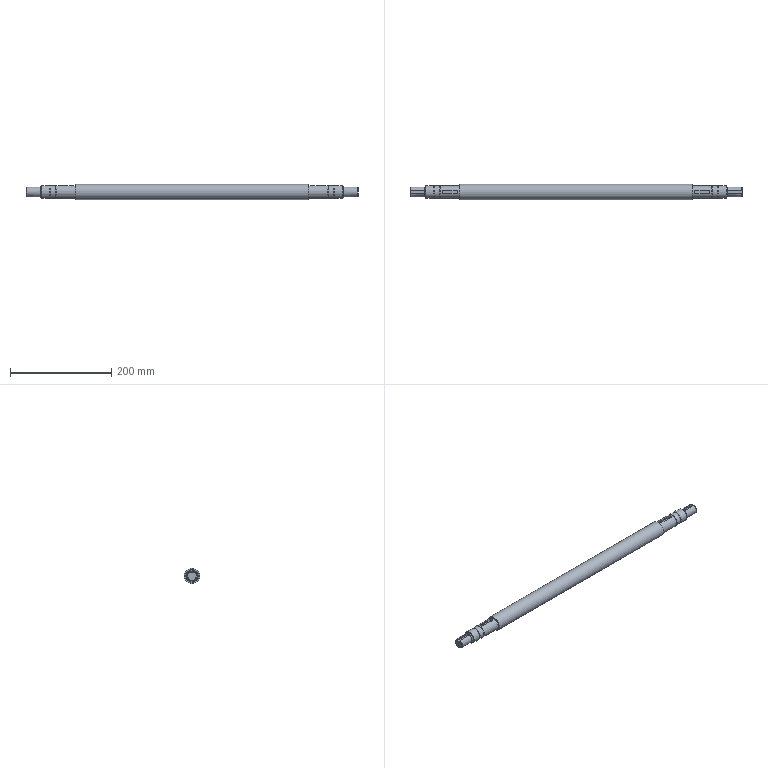Part | 2 solids | 52 faces | box 656 x 30.5 x 30.5 mm | volume 419502 mm3 | plane 27 | cylinder 19 | cone 4 | torus 2 | commonest cylinder face diameters 6 x6 23 x4 25 x4 19.5 x2 25.5 x2 30.5 x1
STEP:
#1=CARTESIAN_POINT('',(-538.673,-3091.93,7.953));
#2=VERTEX_POINT('',#1);
#3=CARTESIAN_POINT('',(-538.673,-3097.93,7.953));
#4=VERTEX_POINT('',#3);
#5=CARTESIAN_POINT('',(-538.673,-3094.93,0.));
#6=DIRECTION('',(-1.,0.,0.));
#7=DIRECTION('',(0.,0.,1.));
#8=AXIS2_PLACEMENT_3D('',#5,#6,#7);
#9=CIRCLE('',#8,8.5);
#10=EDGE_CURVE('',#2,#4,#9,.T.);
#11=ORIENTED_EDGE('',*,*,#10,.T.);
#12=CARTESIAN_POINT('',(-538.673,-3097.93,6.5));
#13=VERTEX_POINT('',#12);
#14=CARTESIAN_POINT('',(-538.673,-3097.93,15.));
#15=DIRECTION('',(0.,0.,-1.));
#16=VECTOR('',#15,1000.);
#17=LINE('',#14,#16);
#18=EDGE_CURVE('',#4,#13,#17,.T.);
#19=ORIENTED_EDGE('',*,*,#18,.T.);
#20=CARTESIAN_POINT('',(-538.673,-3091.93,6.5));
#21=VERTEX_POINT('',#20);
#22=CARTESIAN_POINT('',(-538.673,-3091.93,6.5));
#23=DIRECTION('',(0.,-1.,0.));
#24=VECTOR('',#23,1000.);
#25=LINE('',#22,#24);
#26=EDGE_CURVE('',#21,#13,#25,.T.);
#27=ORIENTED_EDGE('',*,*,#26,.F.);
#28=CARTESIAN_POINT('',(-538.673,-3091.93,15.));
#29=DIRECTION('',(0.,0.,-1.));
#30=VECTOR('',#29,1000.);
#31=LINE('',#28,#30);
#32=EDGE_CURVE('',#2,#21,#31,.T.);
#33=ORIENTED_EDGE('',*,*,#32,.F.);
#34=EDGE_LOOP('',(#11,#19,#27,#33));
#35=FACE_BOUND('',#34,.T.);
#36=CARTESIAN_POINT('',(-538.673,-3086.43,0.));
#37=DIRECTION('',(1.,0.,0.));
#38=DIRECTION('',(0.,0.,-1.));
#39=AXIS2_PLACEMENT_3D('',#36,#37,#38);
#40=PLANE('',#39);
#41=ADVANCED_FACE('',(#35),#40,.F.);
#42=CARTESIAN_POINT('',(-537.423,-3097.93,9.277));
#43=VERTEX_POINT('',#42);
#44=CARTESIAN_POINT('',(-538.673,-3097.93,7.953));
#45=CARTESIAN_POINT('',(-538.258,-3097.93,8.396));
#46=CARTESIAN_POINT('',(-537.842,-3097.93,8.837));
#47=CARTESIAN_POINT('',(-537.423,-3097.93,9.277));
#48=B_SPLINE_CURVE_WITH_KNOTS('',3,(#44,#45,#46,#47),.UNSPECIFIED.,.F.,.F.,(4,4),(0.006081,0.007901),.UNSPECIFIED.);
#49=EDGE_CURVE('',#4,#43,#48,.T.);
#50=ORIENTED_EDGE('',*,*,#49,.F.);
#51=ORIENTED_EDGE('',*,*,#10,.F.);
#52=CARTESIAN_POINT('',(-537.423,-3091.93,9.277));
#53=VERTEX_POINT('',#52);
#54=CARTESIAN_POINT('',(-537.423,-3091.93,9.277));
#55=CARTESIAN_POINT('',(-537.842,-3091.93,8.837));
#56=CARTESIAN_POINT('',(-538.258,-3091.93,8.396));
#57=CARTESIAN_POINT('',(-538.673,-3091.93,7.953));
#58=B_SPLINE_CURVE_WITH_KNOTS('',3,(#54,#55,#56,#57),.UNSPECIFIED.,.F.,.F.,(4,4),(0.004458,0.006278),.UNSPECIFIED.);
#59=EDGE_CURVE('',#53,#2,#58,.T.);
#60=ORIENTED_EDGE('',*,*,#59,.F.);
#61=CARTESIAN_POINT('',(-537.423,-3094.93,0.));
#62=DIRECTION('',(1.,0.,0.));
#63=DIRECTION('',(0.,0.,-1.));
#64=AXIS2_PLACEMENT_3D('',#61,#62,#63);
#65=CIRCLE('',#64,9.75);
#66=EDGE_CURVE('',#53,#43,#65,.F.);
#67=ORIENTED_EDGE('',*,*,#66,.T.);
#68=EDGE_LOOP('',(#50,#51,#60,#67));
#69=FACE_BOUND('',#68,.T.);
#70=CARTESIAN_POINT('',(-537.673,-3094.93,0.));
#71=DIRECTION('',(1.,0.,0.));
#72=DIRECTION('',(0.,0.,-1.));
#73=AXIS2_PLACEMENT_3D('',#70,#71,#72);
#74=CONICAL_SURFACE('',#73,9.5,0.7854);
#75=ADVANCED_FACE('',(#69),#74,.T.);
#76=CARTESIAN_POINT('',(-512.673,-3097.93,9.277));
#77=VERTEX_POINT('',#76);
#78=CARTESIAN_POINT('',(-538.673,-3097.93,9.277));
#79=DIRECTION('',(-1.,0.,0.));
#80=VECTOR('',#79,1000.);
#81=LINE('',#78,#80);
#82=EDGE_CURVE('',#43,#77,#81,.F.);
#83=ORIENTED_EDGE('',*,*,#82,.T.);
#84=CARTESIAN_POINT('',(-512.673,-3097.93,6.5));
#85=VERTEX_POINT('',#84);
#86=CARTESIAN_POINT('',(-512.673,-3097.93,15.));
#87=DIRECTION('',(0.,0.,-1.));
#88=VECTOR('',#87,1000.);
#89=LINE('',#86,#88);
#90=EDGE_CURVE('',#85,#77,#89,.F.);
#91=ORIENTED_EDGE('',*,*,#90,.F.);
#92=CARTESIAN_POINT('',(-538.673,-3097.93,6.5));
#93=DIRECTION('',(1.,0.,0.));
#94=VECTOR('',#93,1000.);
#95=LINE('',#92,#94);
#96=EDGE_CURVE('',#85,#13,#95,.F.);
#97=ORIENTED_EDGE('',*,*,#96,.T.);
#98=ORIENTED_EDGE('',*,*,#18,.F.);
#99=ORIENTED_EDGE('',*,*,#49,.T.);
#100=EDGE_LOOP('',(#83,#91,#97,#98,#99));
#101=FACE_BOUND('',#100,.T.);
#102=CARTESIAN_POINT('',(-538.673,-3097.93,15.));
#103=DIRECTION('',(0.,1.,0.));
#104=DIRECTION('',(0.,0.,1.));
#105=AXIS2_PLACEMENT_3D('',#102,#103,#104);
#106=PLANE('',#105);
#107=ADVANCED_FACE('',(#101),#106,.T.);
#108=ORIENTED_EDGE('',*,*,#26,.T.);
#109=ORIENTED_EDGE('',*,*,#96,.F.);
#110=CARTESIAN_POINT('',(-512.673,-3091.93,6.5));
#111=VERTEX_POINT('',#110);
#112=CARTESIAN_POINT('',(-512.673,-3094.93,6.5));
#113=DIRECTION('',(0.,0.,1.));
#114=DIRECTION('',(1.,0.,0.));
#115=AXIS2_PLACEMENT_3D('',#112,#113,#114);
#116=CIRCLE('',#115,3.);
#117=EDGE_CURVE('',#111,#85,#116,.F.);
#118=ORIENTED_EDGE('',*,*,#117,.F.);
#119=CARTESIAN_POINT('',(-512.673,-3091.93,6.5));
#120=DIRECTION('',(-1.,0.,0.));
#121=VECTOR('',#120,1000.);
#122=LINE('',#119,#121);
#123=EDGE_CURVE('',#21,#111,#122,.F.);
#124=ORIENTED_EDGE('',*,*,#123,.F.);
#125=EDGE_LOOP('',(#108,#109,#118,#124));
#126=FACE_BOUND('',#125,.T.);
#127=CARTESIAN_POINT('',(-512.673,-3094.93,6.5));
#128=DIRECTION('',(0.,0.,1.));
#129=DIRECTION('',(1.,0.,0.));
#130=AXIS2_PLACEMENT_3D('',#127,#128,#129);
#131=PLANE('',#130);
#132=ADVANCED_FACE('',(#126),#131,.T.);
#133=CARTESIAN_POINT('',(-512.673,-3091.93,9.277));
#134=VERTEX_POINT('',#133);
#135=CARTESIAN_POINT('',(-538.673,-3091.93,9.277));
#136=DIRECTION('',(-1.,0.,0.));
#137=VECTOR('',#136,1000.);
#138=LINE('',#135,#137);
#139=EDGE_CURVE('',#134,#53,#138,.T.);
#140=ORIENTED_EDGE('',*,*,#139,.T.);
#141=ORIENTED_EDGE('',*,*,#59,.T.);
#142=ORIENTED_EDGE('',*,*,#32,.T.);
#143=ORIENTED_EDGE('',*,*,#123,.T.);
#144=CARTESIAN_POINT('',(-512.673,-3091.93,15.));
#145=DIRECTION('',(0.,0.,-1.));
#146=VECTOR('',#145,1000.);
#147=LINE('',#144,#146);
#148=EDGE_CURVE('',#111,#134,#147,.F.);
#149=ORIENTED_EDGE('',*,*,#148,.T.);
#150=EDGE_LOOP('',(#140,#141,#142,#143,#149));
#151=FACE_BOUND('',#150,.T.);
#152=CARTESIAN_POINT('',(-512.673,-3091.93,15.));
#153=DIRECTION('',(0.,-1.,0.));
#154=DIRECTION('',(1.,0.,0.));
#155=AXIS2_PLACEMENT_3D('',#152,#153,#154);
#156=PLANE('',#155);
#157=ADVANCED_FACE('',(#151),#156,.T.);
#158=ORIENTED_EDGE('',*,*,#82,.F.);
#159=ORIENTED_EDGE('',*,*,#66,.F.);
#160=ORIENTED_EDGE('',*,*,#139,.F.);
#161=CARTESIAN_POINT('',(-511.002,-3092.438,9.426));
#162=VERTEX_POINT('',#161);
#163=CARTESIAN_POINT('',(-511.002,-3092.438,9.426));
#164=CARTESIAN_POINT('',(-511.488,-3092.112,9.34));
#165=CARTESIAN_POINT('',(-512.083,-3091.93,9.277));
#166=CARTESIAN_POINT('',(-512.673,-3091.93,9.277));
#167=B_SPLINE_CURVE_WITH_KNOTS('',3,(#163,#164,#165,#166),.UNSPECIFIED.,.F.,.F.,(4,4),(0.006723,0.008493),.UNSPECIFIED.);
#168=EDGE_CURVE('',#162,#134,#167,.T.);
#169=ORIENTED_EDGE('',*,*,#168,.F.);
#170=CARTESIAN_POINT('',(-511.002,-3097.421,9.426));
#171=VERTEX_POINT('',#170);
#172=CARTESIAN_POINT('',(-511.002,-3094.93,0.));
#173=DIRECTION('',(1.,0.,0.));
#174=DIRECTION('',(0.,0.,-1.));
#175=AXIS2_PLACEMENT_3D('',#172,#173,#174);
#176=CIRCLE('',#175,9.75);
#177=EDGE_CURVE('',#162,#171,#176,.F.);
#178=ORIENTED_EDGE('',*,*,#177,.T.);
#179=CARTESIAN_POINT('',(-511.002,-3097.421,9.426));
#180=CARTESIAN_POINT('',(-511.488,-3097.747,9.34));
#181=CARTESIAN_POINT('',(-512.083,-3097.93,9.277));
#182=CARTESIAN_POINT('',(-512.673,-3097.93,9.277));
#183=B_SPLINE_CURVE_WITH_KNOTS('',3,(#179,#180,#181,#182),.UNSPECIFIED.,.F.,.F.,(4,4),(0.005694,0.007464),.UNSPECIFIED.);
#184=EDGE_CURVE('',#77,#171,#183,.F.);
#185=ORIENTED_EDGE('',*,*,#184,.F.);
#186=EDGE_LOOP('',(#158,#159,#160,#169,#178,#185));
#187=FACE_BOUND('',#186,.T.);
#188=CARTESIAN_POINT('',(-538.673,-3094.93,0.));
#189=DIRECTION('',(-1.,0.,0.));
#190=DIRECTION('',(0.,0.,1.));
#191=AXIS2_PLACEMENT_3D('',#188,#189,#190);
#192=CYLINDRICAL_SURFACE('',#191,9.75);
#193=ADVANCED_FACE('',(#187),#192,.T.);
#194=ORIENTED_EDGE('',*,*,#168,.T.);
#195=ORIENTED_EDGE('',*,*,#148,.F.);
#196=ORIENTED_EDGE('',*,*,#117,.T.);
#197=ORIENTED_EDGE('',*,*,#90,.T.);
#198=ORIENTED_EDGE('',*,*,#184,.T.);
#199=CARTESIAN_POINT('',(-511.002,-3097.421,9.426));
#200=CARTESIAN_POINT('',(-510.62,-3097.165,9.232));
#201=CARTESIAN_POINT('',(-509.906,-3096.392,9.395));
#202=CARTESIAN_POINT('',(-509.556,-3094.934,9.681));
#203=CARTESIAN_POINT('',(-509.908,-3093.463,9.395));
#204=CARTESIAN_POINT('',(-510.618,-3092.696,9.23));
#205=CARTESIAN_POINT('',(-511.002,-3092.438,9.426));
#206=B_SPLINE_CURVE_WITH_KNOTS('',3,(#199,#200,#201,#202,#203,#204,#205),.UNSPECIFIED.,.F.,.F.,(4,1,1,1,4),(-0.001188,0.0002888,0.001765,0.003242,0.004718),.UNSPECIFIED.);
#207=EDGE_CURVE('',#171,#162,#206,.T.);
#208=ORIENTED_EDGE('',*,*,#207,.T.);
#209=EDGE_LOOP('',(#194,#195,#196,#197,#198,#208));
#210=FACE_BOUND('',#209,.T.);
#211=CARTESIAN_POINT('',(-512.673,-3094.93,15.));
#212=DIRECTION('',(0.,0.,-1.));
#213=DIRECTION('',(-1.,0.,0.));
#214=AXIS2_PLACEMENT_3D('',#211,#212,#213);
#215=CYLINDRICAL_SURFACE('',#214,3.);
#216=ADVANCED_FACE('',(#210),#215,.F.);
#217=CARTESIAN_POINT('',(-508.673,-3094.93,11.));
#218=VERTEX_POINT('',#217);
#219=CARTESIAN_POINT('',(-508.673,-3094.93,0.));
#220=DIRECTION('',(-1.,0.,0.));
#221=DIRECTION('',(0.,0.,1.));
#222=AXIS2_PLACEMENT_3D('',#219,#220,#221);
#223=CIRCLE('',#222,11.);
#224=EDGE_CURVE('',#218,#218,#223,.T.);
#225=ORIENTED_EDGE('',*,*,#224,.T.);
#226=EDGE_LOOP('',(#225));
#227=FACE_BOUND('',#226,.T.);
#228=ORIENTED_EDGE('',*,*,#207,.F.);
#229=ORIENTED_EDGE('',*,*,#177,.F.);
#230=EDGE_LOOP('',(#228,#229));
#231=FACE_BOUND('',#230,.T.);
#232=CARTESIAN_POINT('',(-510.173,-3094.93,0.));
#233=DIRECTION('',(-1.,0.,0.));
#234=DIRECTION('',(0.,0.,1.));
#235=AXIS2_PLACEMENT_3D('',#232,#233,#234);
#236=TOROIDAL_SURFACE('',#235,11.,1.5);
#237=ADVANCED_FACE('',(#227,#231),#236,.F.);
#238=ORIENTED_EDGE('',*,*,#224,.F.);
#239=EDGE_LOOP('',(#238));
#240=FACE_BOUND('',#239,.T.);
#241=CARTESIAN_POINT('',(-508.673,-3094.93,11.5));
#242=VERTEX_POINT('',#241);
#243=CARTESIAN_POINT('',(-508.673,-3094.93,0.));
#244=DIRECTION('',(-1.,0.,0.));
#245=DIRECTION('',(0.,0.,1.));
#246=AXIS2_PLACEMENT_3D('',#243,#244,#245);
#247=CIRCLE('',#246,11.5);
#248=EDGE_CURVE('',#242,#242,#247,.T.);
#249=ORIENTED_EDGE('',*,*,#248,.T.);
#250=EDGE_LOOP('',(#249));
#251=FACE_BOUND('',#250,.T.);
#252=CARTESIAN_POINT('',(-508.673,-3083.43,0.));
#253=DIRECTION('',(1.,0.,0.));
#254=DIRECTION('',(0.,0.,-1.));
#255=AXIS2_PLACEMENT_3D('',#252,#253,#254);
#256=PLANE('',#255);
#257=ADVANCED_FACE('',(#240,#251),#256,.F.);
#258=ORIENTED_EDGE('',*,*,#248,.F.);
#259=EDGE_LOOP('',(#258));
#260=FACE_BOUND('',#259,.T.);
#261=CARTESIAN_POINT('',(-507.673,-3094.93,12.5));
#262=VERTEX_POINT('',#261);
#263=CARTESIAN_POINT('',(-507.673,-3094.93,0.));
#264=DIRECTION('',(-1.,0.,0.));
#265=DIRECTION('',(0.,0.,1.));
#266=AXIS2_PLACEMENT_3D('',#263,#264,#265);
#267=CIRCLE('',#266,12.5);
#268=EDGE_CURVE('',#262,#262,#267,.T.);
#269=ORIENTED_EDGE('',*,*,#268,.T.);
#270=EDGE_LOOP('',(#269));
#271=FACE_BOUND('',#270,.T.);
#272=CARTESIAN_POINT('',(-507.673,-3094.93,0.));
#273=DIRECTION('',(1.,0.,0.));
#274=DIRECTION('',(0.,0.,-1.));
#275=AXIS2_PLACEMENT_3D('',#272,#273,#274);
#276=CONICAL_SURFACE('',#275,12.5,0.7854);
#277=ADVANCED_FACE('',(#260,#271),#276,.T.);
#278=ORIENTED_EDGE('',*,*,#268,.F.);
#279=EDGE_LOOP('',(#278));
#280=FACE_BOUND('',#279,.T.);
#281=CARTESIAN_POINT('',(-492.173,-3094.93,12.5));
#282=VERTEX_POINT('',#281);
#283=CARTESIAN_POINT('',(-492.173,-3094.93,0.));
#284=DIRECTION('',(-1.,0.,0.));
#285=DIRECTION('',(0.,0.,1.));
#286=AXIS2_PLACEMENT_3D('',#283,#284,#285);
#287=CIRCLE('',#286,12.5);
#288=EDGE_CURVE('',#282,#282,#287,.T.);
#289=ORIENTED_EDGE('',*,*,#288,.T.);
#290=EDGE_LOOP('',(#289));
#291=FACE_BOUND('',#290,.T.);
#292=CARTESIAN_POINT('',(-538.673,-3094.93,0.));
#293=DIRECTION('',(-1.,0.,0.));
#294=DIRECTION('',(0.,0.,1.));
#295=AXIS2_PLACEMENT_3D('',#292,#293,#294);
#296=CYLINDRICAL_SURFACE('',#295,12.5);
#297=ADVANCED_FACE('',(#280,#291),#296,.T.);
#298=ORIENTED_EDGE('',*,*,#288,.F.);
#299=EDGE_LOOP('',(#298));
#300=FACE_BOUND('',#299,.T.);
#301=CARTESIAN_POINT('',(-492.173,-3094.93,11.5));
#302=VERTEX_POINT('',#301);
#303=CARTESIAN_POINT('',(-492.173,-3094.93,0.));
#304=DIRECTION('',(-1.,0.,0.));
#305=DIRECTION('',(0.,0.,1.));
#306=AXIS2_PLACEMENT_3D('',#303,#304,#305);
#307=CIRCLE('',#306,11.5);
#308=EDGE_CURVE('',#302,#302,#307,.T.);
#309=ORIENTED_EDGE('',*,*,#308,.T.);
#310=EDGE_LOOP('',(#309));
#311=FACE_BOUND('',#310,.T.);
#312=CARTESIAN_POINT('',(-492.173,-3083.43,0.));
#313=DIRECTION('',(-1.,0.,0.));
#314=DIRECTION('',(0.,0.,1.));
#315=AXIS2_PLACEMENT_3D('',#312,#313,#314);
#316=PLANE('',#315);
#317=ADVANCED_FACE('',(#300,#311),#316,.F.);
#318=ORIENTED_EDGE('',*,*,#308,.F.);
#319=EDGE_LOOP('',(#318));
#320=FACE_BOUND('',#319,.T.);
#321=CARTESIAN_POINT('',(-490.673,-3094.93,11.5));
#322=VERTEX_POINT('',#321);
#323=CARTESIAN_POINT('',(-490.673,-3094.93,0.));
#324=DIRECTION('',(-1.,0.,0.));
#325=DIRECTION('',(0.,0.,1.));
#326=AXIS2_PLACEMENT_3D('',#323,#324,#325);
#327=CIRCLE('',#326,11.5);
#328=EDGE_CURVE('',#322,#322,#327,.T.);
#329=ORIENTED_EDGE('',*,*,#328,.T.);
#330=EDGE_LOOP('',(#329));
#331=FACE_BOUND('',#330,.T.);
#332=CARTESIAN_POINT('',(-538.673,-3094.93,0.));
#333=DIRECTION('',(-1.,0.,0.));
#334=DIRECTION('',(0.,0.,1.));
#335=AXIS2_PLACEMENT_3D('',#332,#333,#334);
#336=CYLINDRICAL_SURFACE('',#335,11.5);
#337=ADVANCED_FACE('',(#320,#331),#336,.T.);
#338=ORIENTED_EDGE('',*,*,#328,.F.);
#339=EDGE_LOOP('',(#338));
#340=FACE_BOUND('',#339,.T.);
#341=CARTESIAN_POINT('',(-490.673,-3094.93,12.5));
#342=VERTEX_POINT('',#341);
#343=CARTESIAN_POINT('',(-490.673,-3094.93,0.));
#344=DIRECTION('',(-1.,0.,0.));
#345=DIRECTION('',(0.,0.,1.));
#346=AXIS2_PLACEMENT_3D('',#343,#344,#345);
#347=CIRCLE('',#346,12.5);
#348=EDGE_CURVE('',#342,#342,#347,.T.);
#349=ORIENTED_EDGE('',*,*,#348,.T.);
#350=EDGE_LOOP('',(#349));
#351=FACE_BOUND('',#350,.T.);
#352=CARTESIAN_POINT('',(-490.673,-3082.43,0.));
#353=DIRECTION('',(1.,0.,0.));
#354=DIRECTION('',(0.,0.,-1.));
#355=AXIS2_PLACEMENT_3D('',#352,#353,#354);
#356=PLANE('',#355);
#357=ADVANCED_FACE('',(#340,#351),#356,.F.);
#358=ORIENTED_EDGE('',*,*,#348,.F.);
#359=EDGE_LOOP('',(#358));
#360=FACE_BOUND('',#359,.T.);
#361=CARTESIAN_POINT('',(-480.673,-3094.93,12.5));
#362=VERTEX_POINT('',#361);
#363=CARTESIAN_POINT('',(-480.673,-3094.93,0.));
#364=DIRECTION('',(-1.,0.,0.));
#365=DIRECTION('',(0.,0.,1.));
#366=AXIS2_PLACEMENT_3D('',#363,#364,#365);
#367=CIRCLE('',#366,12.5);
#368=EDGE_CURVE('',#362,#362,#367,.T.);
#369=ORIENTED_EDGE('',*,*,#368,.T.);
#370=EDGE_LOOP('',(#369));
#371=FACE_BOUND('',#370,.T.);
#372=CARTESIAN_POINT('',(-538.673,-3094.93,0.));
#373=DIRECTION('',(-1.,0.,0.));
#374=DIRECTION('',(0.,0.,1.));
#375=AXIS2_PLACEMENT_3D('',#372,#373,#374);
#376=CYLINDRICAL_SURFACE('',#375,12.5);
#377=ADVANCED_FACE('',(#360,#371),#376,.T.);
#378=ORIENTED_EDGE('',*,*,#368,.F.);
#379=EDGE_LOOP('',(#378));
#380=FACE_BOUND('',#379,.T.);
#381=CARTESIAN_POINT('',(-480.673,-3094.93,11.5));
#382=VERTEX_POINT('',#381);
#383=CARTESIAN_POINT('',(-480.673,-3094.93,0.));
#384=DIRECTION('',(-1.,0.,0.));
#385=DIRECTION('',(0.,0.,1.));
#386=AXIS2_PLACEMENT_3D('',#383,#384,#385);
#387=CIRCLE('',#386,11.5);
#388=EDGE_CURVE('',#382,#382,#387,.T.);
#389=ORIENTED_EDGE('',*,*,#388,.T.);
#390=EDGE_LOOP('',(#389));
#391=FACE_BOUND('',#390,.T.);
#392=CARTESIAN_POINT('',(-480.673,-3083.43,0.));
#393=DIRECTION('',(-1.,0.,0.));
#394=DIRECTION('',(0.,0.,1.));
#395=AXIS2_PLACEMENT_3D('',#392,#393,#394);
#396=PLANE('',#395);
#397=ADVANCED_FACE('',(#380,#391),#396,.F.);
#398=CARTESIAN_POINT('',(-472.423,-3097.93,9.5));
#399=VERTEX_POINT('',#398);
#400=CARTESIAN_POINT('',(-472.423,-3091.93,9.5));
#401=VERTEX_POINT('',#400);
#402=CARTESIAN_POINT('',(-472.423,-3094.93,9.5));
#403=DIRECTION('',(0.,0.,1.));
#404=DIRECTION('',(1.,0.,0.));
#405=AXIS2_PLACEMENT_3D('',#402,#403,#404);
#406=CIRCLE('',#405,3.);
#407=EDGE_CURVE('',#399,#401,#406,.F.);
#408=ORIENTED_EDGE('',*,*,#407,.F.);
#409=CARTESIAN_POINT('',(-447.423,-3097.93,9.5));
#410=VERTEX_POINT('',#409);
#411=CARTESIAN_POINT('',(-472.423,-3097.93,9.5));
#412=DIRECTION('',(1.,0.,0.));
#413=VECTOR('',#412,1000.);
#414=LINE('',#411,#413);
#415=EDGE_CURVE('',#410,#399,#414,.F.);
#416=ORIENTED_EDGE('',*,*,#415,.F.);
#417=CARTESIAN_POINT('',(-447.423,-3091.93,9.5));
#418=VERTEX_POINT('',#417);
#419=CARTESIAN_POINT('',(-447.423,-3094.93,9.5));
#420=DIRECTION('',(0.,0.,1.));
#421=DIRECTION('',(1.,0.,0.));
#422=AXIS2_PLACEMENT_3D('',#419,#420,#421);
#423=CIRCLE('',#422,3.);
#424=EDGE_CURVE('',#418,#410,#423,.F.);
#425=ORIENTED_EDGE('',*,*,#424,.F.);
#426=CARTESIAN_POINT('',(-447.423,-3091.93,9.5));
#427=DIRECTION('',(-1.,0.,0.));
#428=VECTOR('',#427,1000.);
#429=LINE('',#426,#428);
#430=EDGE_CURVE('',#401,#418,#429,.F.);
#431=ORIENTED_EDGE('',*,*,#430,.F.);
#432=EDGE_LOOP('',(#408,#416,#425,#431));
#433=FACE_BOUND('',#432,.T.);
#434=CARTESIAN_POINT('',(-472.423,-3094.93,9.5));
#435=DIRECTION('',(0.,0.,1.));
#436=DIRECTION('',(1.,0.,0.));
#437=AXIS2_PLACEMENT_3D('',#434,#435,#436);
#438=PLANE('',#437);
#439=ADVANCED_FACE('',(#433),#438,.T.);
#440=ORIENTED_EDGE('',*,*,#388,.F.);
#441=EDGE_LOOP('',(#440));
#442=FACE_BOUND('',#441,.T.);
#443=CARTESIAN_POINT('',(-479.173,-3094.93,11.5));
#444=VERTEX_POINT('',#443);
#445=CARTESIAN_POINT('',(-479.173,-3094.93,0.));
#446=DIRECTION('',(-1.,0.,0.));
#447=DIRECTION('',(0.,0.,1.));
#448=AXIS2_PLACEMENT_3D('',#445,#446,#447);
#449=CIRCLE('',#448,11.5);
#450=EDGE_CURVE('',#444,#444,#449,.T.);
#451=ORIENTED_EDGE('',*,*,#450,.T.);
#452=EDGE_LOOP('',(#451));
#453=FACE_BOUND('',#452,.T.);
#454=CARTESIAN_POINT('',(-538.673,-3094.93,0.));
#455=DIRECTION('',(-1.,0.,0.));
#456=DIRECTION('',(0.,0.,1.));
#457=AXIS2_PLACEMENT_3D('',#454,#455,#456);
#458=CYLINDRICAL_SURFACE('',#457,11.5);
#459=ADVANCED_FACE('',(#442,#453),#458,.T.);
#460=CARTESIAN_POINT('',(-472.423,-3097.93,12.392));
#461=VERTEX_POINT('',#460);
#462=CARTESIAN_POINT('',(-447.423,-3097.93,12.392));
#463=VERTEX_POINT('',#462);
#464=CARTESIAN_POINT('',(-538.673,-3097.93,12.392));
#465=DIRECTION('',(-1.,0.,0.));
#466=VECTOR('',#465,1000.);
#467=LINE('',#464,#466);
#468=EDGE_CURVE('',#461,#463,#467,.F.);
#469=ORIENTED_EDGE('',*,*,#468,.T.);
#470=CARTESIAN_POINT('',(-447.423,-3097.93,15.));
#471=DIRECTION('',(0.,0.,-1.));
#472=VECTOR('',#471,1000.);
#473=LINE('',#470,#472);
#474=EDGE_CURVE('',#410,#463,#473,.F.);
#475=ORIENTED_EDGE('',*,*,#474,.F.);
#476=ORIENTED_EDGE('',*,*,#415,.T.);
#477=CARTESIAN_POINT('',(-472.423,-3097.93,15.));
#478=DIRECTION('',(0.,0.,-1.));
#479=VECTOR('',#478,1000.);
#480=LINE('',#477,#479);
#481=EDGE_CURVE('',#399,#461,#480,.F.);
#482=ORIENTED_EDGE('',*,*,#481,.T.);
#483=EDGE_LOOP('',(#469,#475,#476,#482));
#484=FACE_BOUND('',#483,.T.);
#485=CARTESIAN_POINT('',(-472.423,-3097.93,15.));
#486=DIRECTION('',(0.,1.,0.));
#487=DIRECTION('',(0.,0.,1.));
#488=AXIS2_PLACEMENT_3D('',#485,#486,#487);
#489=PLANE('',#488);
#490=ADVANCED_FACE('',(#484),#489,.T.);
#491=CARTESIAN_POINT('',(-447.423,-3091.93,12.392));
#492=VERTEX_POINT('',#491);
#493=CARTESIAN_POINT('',(-447.423,-3097.93,12.392));
#494=CARTESIAN_POINT('',(-446.636,-3097.93,12.392));
#495=CARTESIAN_POINT('',(-445.072,-3097.279,12.574));
#496=CARTESIAN_POINT('',(-444.098,-3094.93,12.838));
#497=CARTESIAN_POINT('',(-445.075,-3092.577,12.573));
#498=CARTESIAN_POINT('',(-446.638,-3091.93,12.392));
#499=CARTESIAN_POINT('',(-447.423,-3091.93,12.392));
#500=B_SPLINE_CURVE_WITH_KNOTS('',3,(#493,#494,#495,#496,#497,#498,#499),.UNSPECIFIED.,.F.,.F.,(4,1,1,1,4),(0.01381,0.01616,0.01851,0.02086,0.02322),.UNSPECIFIED.);
#501=EDGE_CURVE('',#463,#492,#500,.T.);
#502=ORIENTED_EDGE('',*,*,#501,.T.);
#503=CARTESIAN_POINT('',(-447.423,-3091.93,15.));
#504=DIRECTION('',(0.,0.,-1.));
#505=VECTOR('',#504,1000.);
#506=LINE('',#503,#505);
#507=EDGE_CURVE('',#418,#492,#506,.F.);
#508=ORIENTED_EDGE('',*,*,#507,.F.);
#509=ORIENTED_EDGE('',*,*,#424,.T.);
#510=ORIENTED_EDGE('',*,*,#474,.T.);
#511=EDGE_LOOP('',(#502,#508,#509,#510));
#512=FACE_BOUND('',#511,.T.);
#513=CARTESIAN_POINT('',(-447.423,-3094.93,15.));
#514=DIRECTION('',(0.,0.,-1.));
#515=DIRECTION('',(-1.,0.,0.));
#516=AXIS2_PLACEMENT_3D('',#513,#514,#515);
#517=CYLINDRICAL_SURFACE('',#516,3.);
#518=ADVANCED_FACE('',(#512),#517,.F.);
#519=CARTESIAN_POINT('',(-472.423,-3091.93,12.392));
#520=VERTEX_POINT('',#519);
#521=CARTESIAN_POINT('',(-447.423,-3091.93,12.392));
#522=DIRECTION('',(-1.,0.,0.));
#523=VECTOR('',#522,1000.);
#524=LINE('',#521,#523);
#525=EDGE_CURVE('',#492,#520,#524,.T.);
#526=ORIENTED_EDGE('',*,*,#525,.T.);
#527=CARTESIAN_POINT('',(-472.423,-3091.93,15.));
#528=DIRECTION('',(0.,0.,-1.));
#529=VECTOR('',#528,1000.);
#530=LINE('',#527,#529);
#531=EDGE_CURVE('',#401,#520,#530,.F.);
#532=ORIENTED_EDGE('',*,*,#531,.F.);
#533=ORIENTED_EDGE('',*,*,#430,.T.);
#534=ORIENTED_EDGE('',*,*,#507,.T.);
#535=EDGE_LOOP('',(#526,#532,#533,#534));
#536=FACE_BOUND('',#535,.T.);
#537=CARTESIAN_POINT('',(-447.423,-3091.93,15.));
#538=DIRECTION('',(0.,-1.,0.));
#539=DIRECTION('',(0.,0.,-1.));
#540=AXIS2_PLACEMENT_3D('',#537,#538,#539);
#541=PLANE('',#540);
#542=ADVANCED_FACE('',(#536),#541,.T.);
#543=CARTESIAN_POINT('',(-472.423,-3091.93,12.392));
#544=CARTESIAN_POINT('',(-473.217,-3091.93,12.392));
#545=CARTESIAN_POINT('',(-474.771,-3092.581,12.574));
#546=CARTESIAN_POINT('',(-475.749,-3094.928,12.838));
#547=CARTESIAN_POINT('',(-474.772,-3097.282,12.573));
#548=CARTESIAN_POINT('',(-473.208,-3097.93,12.392));
#549=CARTESIAN_POINT('',(-472.423,-3097.93,12.392));
#550=B_SPLINE_CURVE_WITH_KNOTS('',3,(#543,#544,#545,#546,#547,#548,#549),.UNSPECIFIED.,.F.,.F.,(4,1,1,1,4),(0.001956,0.004309,0.006662,0.009016,0.01137),.UNSPECIFIED.);
#551=EDGE_CURVE('',#520,#461,#550,.T.);
#552=ORIENTED_EDGE('',*,*,#551,.T.);
#553=ORIENTED_EDGE('',*,*,#481,.F.);
#554=ORIENTED_EDGE('',*,*,#407,.T.);
#555=ORIENTED_EDGE('',*,*,#531,.T.);
#556=EDGE_LOOP('',(#552,#553,#554,#555));
#557=FACE_BOUND('',#556,.T.);
#558=CARTESIAN_POINT('',(-472.423,-3094.93,15.));
#559=DIRECTION('',(0.,0.,-1.));
#560=DIRECTION('',(-1.,0.,0.));
#561=AXIS2_PLACEMENT_3D('',#558,#559,#560);
#562=CYLINDRICAL_SURFACE('',#561,3.);
#563=ADVANCED_FACE('',(#557),#562,.F.);
#564=ORIENTED_EDGE('',*,*,#450,.F.);
#565=EDGE_LOOP('',(#564));
#566=FACE_BOUND('',#565,.T.);
#567=CARTESIAN_POINT('',(-479.173,-3094.93,-12.75));
#568=VERTEX_POINT('',#567);
#569=CARTESIAN_POINT('',(-479.173,-3094.93,0.));
#570=DIRECTION('',(1.,0.,0.));
#571=DIRECTION('',(0.,0.,-1.));
#572=AXIS2_PLACEMENT_3D('',#569,#570,#571);
#573=CIRCLE('',#572,12.75);
#574=EDGE_CURVE('',#568,#568,#573,.F.);
#575=ORIENTED_EDGE('',*,*,#574,.T.);
#576=EDGE_LOOP('',(#575));
#577=FACE_BOUND('',#576,.T.);
#578=CARTESIAN_POINT('',(-479.173,-3082.43,0.));
#579=DIRECTION('',(1.,0.,0.));
#580=DIRECTION('',(0.,0.,-1.));
#581=AXIS2_PLACEMENT_3D('',#578,#579,#580);
#582=PLANE('',#581);
#583=ADVANCED_FACE('',(#566,#577),#582,.F.);
#584=CARTESIAN_POINT('',(-440.673,-3094.93,12.75));
#585=VERTEX_POINT('',#584);
#586=CARTESIAN_POINT('',(-440.673,-3094.93,0.));
#587=DIRECTION('',(-1.,0.,0.));
#588=DIRECTION('',(0.,0.,1.));
#589=AXIS2_PLACEMENT_3D('',#586,#587,#588);
#590=CIRCLE('',#589,12.75);
#591=EDGE_CURVE('',#585,#585,#590,.T.);
#592=ORIENTED_EDGE('',*,*,#591,.T.);
#593=EDGE_LOOP('',(#592));
#594=FACE_BOUND('',#593,.T.);
#595=ORIENTED_EDGE('',*,*,#574,.F.);
#596=EDGE_LOOP('',(#595));
#597=FACE_BOUND('',#596,.T.);
#598=ORIENTED_EDGE('',*,*,#551,.F.);
#599=ORIENTED_EDGE('',*,*,#525,.F.);
#600=ORIENTED_EDGE('',*,*,#501,.F.);
#601=ORIENTED_EDGE('',*,*,#468,.F.);
#602=EDGE_LOOP('',(#598,#599,#600,#601));
#603=FACE_BOUND('',#602,.T.);
#604=CARTESIAN_POINT('',(-538.673,-3094.93,0.));
#605=DIRECTION('',(-1.,0.,0.));
#606=DIRECTION('',(0.,0.,1.));
#607=AXIS2_PLACEMENT_3D('',#604,#605,#606);
#608=CYLINDRICAL_SURFACE('',#607,12.75);
#609=ADVANCED_FACE('',(#594,#597,#603),#608,.T.);
#610=ORIENTED_EDGE('',*,*,#591,.F.);
#611=EDGE_LOOP('',(#610));
#612=FACE_BOUND('',#611,.T.);
#613=CARTESIAN_POINT('',(-440.673,-3094.93,0.));
#614=DIRECTION('',(-1.,0.,0.));
#615=DIRECTION('',(0.,0.,1.));
#616=AXIS2_PLACEMENT_3D('',#613,#614,#615);
#617=PLANE('',#616);
#618=ADVANCED_FACE('',(#612),#617,.F.);
#619=CLOSED_SHELL('',(#41,#75,#107,#132,#157,#193,#216,#237,#257,#277,#297,#317,#337,#357,#377,#397,#439,#459,#490,#518,#542,#563,#583,#609,#618));
#620=MANIFOLD_SOLID_BREP('',#619);
#621=CARTESIAN_POINT('',(117.327,-3091.93,7.953));
#622=VERTEX_POINT('',#621);
#623=CARTESIAN_POINT('',(116.077,-3091.93,9.277));
#624=VERTEX_POINT('',#623);
#625=CARTESIAN_POINT('',(117.327,-3091.93,7.953));
#626=CARTESIAN_POINT('',(116.912,-3091.93,8.396));
#627=CARTESIAN_POINT('',(116.495,-3091.93,8.837));
#628=CARTESIAN_POINT('',(116.077,-3091.93,9.277));
#629=B_SPLINE_CURVE_WITH_KNOTS('',3,(#625,#626,#627,#628),.UNSPECIFIED.,.F.,.F.,(4,4),(0.006081,0.007901),.UNSPECIFIED.);
#630=EDGE_CURVE('',#622,#624,#629,.T.);
#631=ORIENTED_EDGE('',*,*,#630,.F.);
#632=CARTESIAN_POINT('',(117.327,-3097.93,7.953));
#633=VERTEX_POINT('',#632);
#634=CARTESIAN_POINT('',(117.327,-3094.93,0.));
#635=DIRECTION('',(-1.,0.,0.));
#636=DIRECTION('',(0.,0.,1.));
#637=AXIS2_PLACEMENT_3D('',#634,#635,#636);
#638=CIRCLE('',#637,8.5);
#639=EDGE_CURVE('',#622,#633,#638,.T.);
#640=ORIENTED_EDGE('',*,*,#639,.T.);
#641=CARTESIAN_POINT('',(116.077,-3097.93,9.277));
#642=VERTEX_POINT('',#641);
#643=CARTESIAN_POINT('',(116.077,-3097.93,9.277));
#644=CARTESIAN_POINT('',(116.495,-3097.93,8.837));
#645=CARTESIAN_POINT('',(116.912,-3097.93,8.396));
#646=CARTESIAN_POINT('',(117.327,-3097.93,7.953));
#647=B_SPLINE_CURVE_WITH_KNOTS('',3,(#643,#644,#645,#646),.UNSPECIFIED.,.F.,.F.,(4,4),(0.004458,0.006278),.UNSPECIFIED.);
#648=EDGE_CURVE('',#642,#633,#647,.T.);
#649=ORIENTED_EDGE('',*,*,#648,.F.);
#650=CARTESIAN_POINT('',(116.077,-3094.93,0.));
#651=DIRECTION('',(-1.,0.,0.));
#652=DIRECTION('',(0.,0.,1.));
#653=AXIS2_PLACEMENT_3D('',#650,#651,#652);
#654=CIRCLE('',#653,9.75);
#655=EDGE_CURVE('',#624,#642,#654,.T.);
#656=ORIENTED_EDGE('',*,*,#655,.F.);
#657=EDGE_LOOP('',(#631,#640,#649,#656));
#658=FACE_BOUND('',#657,.T.);
#659=CARTESIAN_POINT('',(117.327,-3094.93,0.));
#660=DIRECTION('',(-1.,0.,0.));
#661=DIRECTION('',(0.,0.,1.));
#662=AXIS2_PLACEMENT_3D('',#659,#660,#661);
#663=CONICAL_SURFACE('',#662,8.5,0.7854);
#664=ADVANCED_FACE('',(#658),#663,.T.);
#665=CARTESIAN_POINT('',(91.327,-3091.93,9.277));
#666=VERTEX_POINT('',#665);
#667=CARTESIAN_POINT('',(-141.136,-3091.93,9.277));
#668=DIRECTION('',(-1.,0.,0.));
#669=VECTOR('',#668,1000.);
#670=LINE('',#667,#669);
#671=EDGE_CURVE('',#624,#666,#670,.T.);
#672=ORIENTED_EDGE('',*,*,#671,.F.);
#673=ORIENTED_EDGE('',*,*,#655,.T.);
#674=CARTESIAN_POINT('',(91.327,-3097.93,9.277));
#675=VERTEX_POINT('',#674);
#676=CARTESIAN_POINT('',(-141.136,-3097.93,9.277));
#677=DIRECTION('',(-1.,0.,0.));
#678=VECTOR('',#677,1000.);
#679=LINE('',#676,#678);
#680=EDGE_CURVE('',#675,#642,#679,.F.);
#681=ORIENTED_EDGE('',*,*,#680,.F.);
#682=CARTESIAN_POINT('',(89.656,-3097.421,9.426));
#683=VERTEX_POINT('',#682);
#684=CARTESIAN_POINT('',(89.656,-3097.421,9.426));
#685=CARTESIAN_POINT('',(90.142,-3097.747,9.34));
#686=CARTESIAN_POINT('',(90.737,-3097.93,9.277));
#687=CARTESIAN_POINT('',(91.327,-3097.93,9.277));
#688=B_SPLINE_CURVE_WITH_KNOTS('',3,(#684,#685,#686,#687),.UNSPECIFIED.,.F.,.F.,(4,4),(0.006723,0.008493),.UNSPECIFIED.);
#689=EDGE_CURVE('',#683,#675,#688,.T.);
#690=ORIENTED_EDGE('',*,*,#689,.F.);
#691=CARTESIAN_POINT('',(89.656,-3092.438,9.426));
#692=VERTEX_POINT('',#691);
#693=CARTESIAN_POINT('',(89.656,-3094.93,0.));
#694=DIRECTION('',(-1.,0.,0.));
#695=DIRECTION('',(0.,0.,1.));
#696=AXIS2_PLACEMENT_3D('',#693,#694,#695);
#697=CIRCLE('',#696,9.75);
#698=EDGE_CURVE('',#692,#683,#697,.T.);
#699=ORIENTED_EDGE('',*,*,#698,.F.);
#700=CARTESIAN_POINT('',(89.656,-3092.438,9.426));
#701=CARTESIAN_POINT('',(90.142,-3092.112,9.34));
#702=CARTESIAN_POINT('',(90.737,-3091.93,9.277));
#703=CARTESIAN_POINT('',(91.327,-3091.93,9.277));
#704=B_SPLINE_CURVE_WITH_KNOTS('',3,(#700,#701,#702,#703),.UNSPECIFIED.,.F.,.F.,(4,4),(0.005694,0.007464),.UNSPECIFIED.);
#705=EDGE_CURVE('',#666,#692,#704,.F.);
#706=ORIENTED_EDGE('',*,*,#705,.F.);
#707=EDGE_LOOP('',(#672,#673,#681,#690,#699,#706));
#708=FACE_BOUND('',#707,.T.);
#709=CARTESIAN_POINT('',(-141.136,-3094.93,0.));
#710=DIRECTION('',(-1.,0.,0.));
#711=DIRECTION('',(0.,0.,1.));
#712=AXIS2_PLACEMENT_3D('',#709,#710,#711);
#713=CYLINDRICAL_SURFACE('',#712,9.75);
#714=ADVANCED_FACE('',(#708),#713,.T.);
#715=CARTESIAN_POINT('',(87.327,-3094.93,11.));
#716=VERTEX_POINT('',#715);
#717=CARTESIAN_POINT('',(87.327,-3094.93,0.));
#718=DIRECTION('',(-1.,0.,0.));
#719=DIRECTION('',(0.,0.,1.));
#720=AXIS2_PLACEMENT_3D('',#717,#718,#719);
#721=CIRCLE('',#720,11.);
#722=EDGE_CURVE('',#716,#716,#721,.T.);
#723=ORIENTED_EDGE('',*,*,#722,.F.);
#724=EDGE_LOOP('',(#723));
#725=FACE_BOUND('',#724,.T.);
#726=CARTESIAN_POINT('',(89.656,-3092.438,9.426));
#727=CARTESIAN_POINT('',(89.274,-3092.695,9.232));
#728=CARTESIAN_POINT('',(88.56,-3093.468,9.395));
#729=CARTESIAN_POINT('',(88.21,-3094.926,9.681));
#730=CARTESIAN_POINT('',(88.562,-3096.396,9.395));
#731=CARTESIAN_POINT('',(89.271,-3097.163,9.23));
#732=CARTESIAN_POINT('',(89.656,-3097.421,9.426));
#733=B_SPLINE_CURVE_WITH_KNOTS('',3,(#726,#727,#728,#729,#730,#731,#732),.UNSPECIFIED.,.F.,.F.,(4,1,1,1,4),(-0.001188,0.0002888,0.001765,0.003242,0.004718),.UNSPECIFIED.);
#734=EDGE_CURVE('',#692,#683,#733,.T.);
#735=ORIENTED_EDGE('',*,*,#734,.F.);
#736=ORIENTED_EDGE('',*,*,#698,.T.);
#737=EDGE_LOOP('',(#735,#736));
#738=FACE_BOUND('',#737,.T.);
#739=CARTESIAN_POINT('',(88.827,-3094.93,0.));
#740=DIRECTION('',(-1.,0.,0.));
#741=DIRECTION('',(0.,0.,1.));
#742=AXIS2_PLACEMENT_3D('',#739,#740,#741);
#743=TOROIDAL_SURFACE('',#742,11.,1.5);
#744=ADVANCED_FACE('',(#725,#738),#743,.F.);
#745=ORIENTED_EDGE('',*,*,#639,.F.);
#746=CARTESIAN_POINT('',(117.327,-3091.93,6.5));
#747=VERTEX_POINT('',#746);
#748=CARTESIAN_POINT('',(117.327,-3091.93,15.));
#749=DIRECTION('',(0.,0.,-1.));
#750=VECTOR('',#749,1000.);
#751=LINE('',#748,#750);
#752=EDGE_CURVE('',#622,#747,#751,.T.);
#753=ORIENTED_EDGE('',*,*,#752,.T.);
#754=CARTESIAN_POINT('',(117.327,-3097.93,6.5));
#755=VERTEX_POINT('',#754);
#756=CARTESIAN_POINT('',(117.327,-3097.93,6.5));
#757=DIRECTION('',(0.,1.,0.));
#758=VECTOR('',#757,1000.);
#759=LINE('',#756,#758);
#760=EDGE_CURVE('',#755,#747,#759,.T.);
#761=ORIENTED_EDGE('',*,*,#760,.F.);
#762=CARTESIAN_POINT('',(117.327,-3097.93,15.));
#763=DIRECTION('',(0.,0.,-1.));
#764=VECTOR('',#763,1000.);
#765=LINE('',#762,#764);
#766=EDGE_CURVE('',#633,#755,#765,.T.);
#767=ORIENTED_EDGE('',*,*,#766,.F.);
#768=EDGE_LOOP('',(#745,#753,#761,#767));
#769=FACE_BOUND('',#768,.T.);
#770=CARTESIAN_POINT('',(117.327,-3094.93,0.));
#771=DIRECTION('',(-1.,0.,0.));
#772=DIRECTION('',(0.,0.,1.));
#773=AXIS2_PLACEMENT_3D('',#770,#771,#772);
#774=PLANE('',#773);
#775=ADVANCED_FACE('',(#769),#774,.F.);
#776=CARTESIAN_POINT('',(87.327,-3094.93,11.5));
#777=VERTEX_POINT('',#776);
#778=CARTESIAN_POINT('',(87.327,-3094.93,0.));
#779=DIRECTION('',(-1.,0.,0.));
#780=DIRECTION('',(0.,0.,1.));
#781=AXIS2_PLACEMENT_3D('',#778,#779,#780);
#782=CIRCLE('',#781,11.5);
#783=EDGE_CURVE('',#777,#777,#782,.T.);
#784=ORIENTED_EDGE('',*,*,#783,.F.);
#785=EDGE_LOOP('',(#784));
#786=FACE_BOUND('',#785,.T.);
#787=ORIENTED_EDGE('',*,*,#722,.T.);
#788=EDGE_LOOP('',(#787));
#789=FACE_BOUND('',#788,.T.);
#790=CARTESIAN_POINT('',(87.327,-3083.93,0.));
#791=DIRECTION('',(-1.,0.,0.));
#792=DIRECTION('',(0.,0.,1.));
#793=AXIS2_PLACEMENT_3D('',#790,#791,#792);
#794=PLANE('',#793);
#795=ADVANCED_FACE('',(#786,#789),#794,.F.);
#796=CARTESIAN_POINT('',(86.327,-3094.93,12.5));
#797=VERTEX_POINT('',#796);
#798=CARTESIAN_POINT('',(86.327,-3094.93,0.));
#799=DIRECTION('',(-1.,0.,0.));
#800=DIRECTION('',(0.,0.,1.));
#801=AXIS2_PLACEMENT_3D('',#798,#799,#800);
#802=CIRCLE('',#801,12.5);
#803=EDGE_CURVE('',#797,#797,#802,.T.);
#804=ORIENTED_EDGE('',*,*,#803,.F.);
#805=EDGE_LOOP('',(#804));
#806=FACE_BOUND('',#805,.T.);
#807=ORIENTED_EDGE('',*,*,#783,.T.);
#808=EDGE_LOOP('',(#807));
#809=FACE_BOUND('',#808,.T.);
#810=CARTESIAN_POINT('',(87.327,-3094.93,0.));
#811=DIRECTION('',(-1.,0.,0.));
#812=DIRECTION('',(0.,0.,1.));
#813=AXIS2_PLACEMENT_3D('',#810,#811,#812);
#814=CONICAL_SURFACE('',#813,11.5,0.7854);
#815=ADVANCED_FACE('',(#806,#809),#814,.T.);
#816=CARTESIAN_POINT('',(70.827,-3094.93,12.5));
#817=VERTEX_POINT('',#816);
#818=CARTESIAN_POINT('',(70.827,-3094.93,0.));
#819=DIRECTION('',(-1.,0.,0.));
#820=DIRECTION('',(0.,0.,1.));
#821=AXIS2_PLACEMENT_3D('',#818,#819,#820);
#822=CIRCLE('',#821,12.5);
#823=EDGE_CURVE('',#817,#817,#822,.T.);
#824=ORIENTED_EDGE('',*,*,#823,.F.);
#825=EDGE_LOOP('',(#824));
#826=FACE_BOUND('',#825,.T.);
#827=ORIENTED_EDGE('',*,*,#803,.T.);
#828=EDGE_LOOP('',(#827));
#829=FACE_BOUND('',#828,.T.);
#830=CARTESIAN_POINT('',(-141.136,-3094.93,0.));
#831=DIRECTION('',(-1.,0.,0.));
#832=DIRECTION('',(0.,0.,1.));
#833=AXIS2_PLACEMENT_3D('',#830,#831,#832);
#834=CYLINDRICAL_SURFACE('',#833,12.5);
#835=ADVANCED_FACE('',(#826,#829),#834,.T.);
#836=CARTESIAN_POINT('',(70.827,-3094.93,11.5));
#837=VERTEX_POINT('',#836);
#838=CARTESIAN_POINT('',(70.827,-3094.93,0.));
#839=DIRECTION('',(-1.,0.,0.));
#840=DIRECTION('',(0.,0.,1.));
#841=AXIS2_PLACEMENT_3D('',#838,#839,#840);
#842=CIRCLE('',#841,11.5);
#843=EDGE_CURVE('',#837,#837,#842,.T.);
#844=ORIENTED_EDGE('',*,*,#843,.F.);
#845=EDGE_LOOP('',(#844));
#846=FACE_BOUND('',#845,.T.);
#847=ORIENTED_EDGE('',*,*,#823,.T.);
#848=EDGE_LOOP('',(#847));
#849=FACE_BOUND('',#848,.T.);
#850=CARTESIAN_POINT('',(70.827,-3082.43,0.));
#851=DIRECTION('',(1.,0.,0.));
#852=DIRECTION('',(0.,0.,-1.));
#853=AXIS2_PLACEMENT_3D('',#850,#851,#852);
#854=PLANE('',#853);
#855=ADVANCED_FACE('',(#846,#849),#854,.F.);
#856=CARTESIAN_POINT('',(69.327,-3094.93,11.5));
#857=VERTEX_POINT('',#856);
#858=CARTESIAN_POINT('',(69.327,-3094.93,0.));
#859=DIRECTION('',(-1.,0.,0.));
#860=DIRECTION('',(0.,0.,1.));
#861=AXIS2_PLACEMENT_3D('',#858,#859,#860);
#862=CIRCLE('',#861,11.5);
#863=EDGE_CURVE('',#857,#857,#862,.T.);
#864=ORIENTED_EDGE('',*,*,#863,.F.);
#865=EDGE_LOOP('',(#864));
#866=FACE_BOUND('',#865,.T.);
#867=ORIENTED_EDGE('',*,*,#843,.T.);
#868=EDGE_LOOP('',(#867));
#869=FACE_BOUND('',#868,.T.);
#870=CARTESIAN_POINT('',(-141.136,-3094.93,0.));
#871=DIRECTION('',(-1.,0.,0.));
#872=DIRECTION('',(0.,0.,1.));
#873=AXIS2_PLACEMENT_3D('',#870,#871,#872);
#874=CYLINDRICAL_SURFACE('',#873,11.5);
#875=ADVANCED_FACE('',(#866,#869),#874,.T.);
#876=CARTESIAN_POINT('',(69.327,-3094.93,12.5));
#877=VERTEX_POINT('',#876);
#878=CARTESIAN_POINT('',(69.327,-3094.93,0.));
#879=DIRECTION('',(-1.,0.,0.));
#880=DIRECTION('',(0.,0.,1.));
#881=AXIS2_PLACEMENT_3D('',#878,#879,#880);
#882=CIRCLE('',#881,12.5);
#883=EDGE_CURVE('',#877,#877,#882,.T.);
#884=ORIENTED_EDGE('',*,*,#883,.F.);
#885=EDGE_LOOP('',(#884));
#886=FACE_BOUND('',#885,.T.);
#887=ORIENTED_EDGE('',*,*,#863,.T.);
#888=EDGE_LOOP('',(#887));
#889=FACE_BOUND('',#888,.T.);
#890=CARTESIAN_POINT('',(69.327,-3083.43,0.));
#891=DIRECTION('',(-1.,0.,0.));
#892=DIRECTION('',(0.,0.,1.));
#893=AXIS2_PLACEMENT_3D('',#890,#891,#892);
#894=PLANE('',#893);
#895=ADVANCED_FACE('',(#886,#889),#894,.F.);
#896=CARTESIAN_POINT('',(59.327,-3094.93,12.5));
#897=VERTEX_POINT('',#896);
#898=CARTESIAN_POINT('',(59.327,-3094.93,0.));
#899=DIRECTION('',(-1.,0.,0.));
#900=DIRECTION('',(0.,0.,1.));
#901=AXIS2_PLACEMENT_3D('',#898,#899,#900);
#902=CIRCLE('',#901,12.5);
#903=EDGE_CURVE('',#897,#897,#902,.T.);
#904=ORIENTED_EDGE('',*,*,#903,.F.);
#905=EDGE_LOOP('',(#904));
#906=FACE_BOUND('',#905,.T.);
#907=ORIENTED_EDGE('',*,*,#883,.T.);
#908=EDGE_LOOP('',(#907));
#909=FACE_BOUND('',#908,.T.);
#910=CARTESIAN_POINT('',(-141.136,-3094.93,0.));
#911=DIRECTION('',(-1.,0.,0.));
#912=DIRECTION('',(0.,0.,1.));
#913=AXIS2_PLACEMENT_3D('',#910,#911,#912);
#914=CYLINDRICAL_SURFACE('',#913,12.5);
#915=ADVANCED_FACE('',(#906,#909),#914,.T.);
#916=CARTESIAN_POINT('',(59.327,-3094.93,11.5));
#917=VERTEX_POINT('',#916);
#918=CARTESIAN_POINT('',(59.327,-3094.93,0.));
#919=DIRECTION('',(-1.,0.,0.));
#920=DIRECTION('',(0.,0.,1.));
#921=AXIS2_PLACEMENT_3D('',#918,#919,#920);
#922=CIRCLE('',#921,11.5);
#923=EDGE_CURVE('',#917,#917,#922,.T.);
#924=ORIENTED_EDGE('',*,*,#923,.F.);
#925=EDGE_LOOP('',(#924));
#926=FACE_BOUND('',#925,.T.);
#927=ORIENTED_EDGE('',*,*,#903,.T.);
#928=EDGE_LOOP('',(#927));
#929=FACE_BOUND('',#928,.T.);
#930=CARTESIAN_POINT('',(59.327,-3082.43,0.));
#931=DIRECTION('',(1.,0.,0.));
#932=DIRECTION('',(0.,0.,-1.));
#933=AXIS2_PLACEMENT_3D('',#930,#931,#932);
#934=PLANE('',#933);
#935=ADVANCED_FACE('',(#926,#929),#934,.F.);
#936=CARTESIAN_POINT('',(57.827,-3094.93,11.5));
#937=VERTEX_POINT('',#936);
#938=CARTESIAN_POINT('',(57.827,-3094.93,0.));
#939=DIRECTION('',(-1.,0.,0.));
#940=DIRECTION('',(0.,0.,1.));
#941=AXIS2_PLACEMENT_3D('',#938,#939,#940);
#942=CIRCLE('',#941,11.5);
#943=EDGE_CURVE('',#937,#937,#942,.T.);
#944=ORIENTED_EDGE('',*,*,#943,.F.);
#945=EDGE_LOOP('',(#944));
#946=FACE_BOUND('',#945,.T.);
#947=ORIENTED_EDGE('',*,*,#923,.T.);
#948=EDGE_LOOP('',(#947));
#949=FACE_BOUND('',#948,.T.);
#950=CARTESIAN_POINT('',(-141.136,-3094.93,0.));
#951=DIRECTION('',(-1.,0.,0.));
#952=DIRECTION('',(0.,0.,1.));
#953=AXIS2_PLACEMENT_3D('',#950,#951,#952);
#954=CYLINDRICAL_SURFACE('',#953,11.5);
#955=ADVANCED_FACE('',(#946,#949),#954,.T.);
#956=CARTESIAN_POINT('',(57.827,-3094.93,12.75));
#957=VERTEX_POINT('',#956);
#958=CARTESIAN_POINT('',(57.827,-3094.93,0.));
#959=DIRECTION('',(-1.,0.,0.));
#960=DIRECTION('',(0.,0.,1.));
#961=AXIS2_PLACEMENT_3D('',#958,#959,#960);
#962=CIRCLE('',#961,12.75);
#963=EDGE_CURVE('',#957,#957,#962,.T.);
#964=ORIENTED_EDGE('',*,*,#963,.F.);
#965=EDGE_LOOP('',(#964));
#966=FACE_BOUND('',#965,.T.);
#967=ORIENTED_EDGE('',*,*,#943,.T.);
#968=EDGE_LOOP('',(#967));
#969=FACE_BOUND('',#968,.T.);
#970=CARTESIAN_POINT('',(57.827,-3083.43,0.));
#971=DIRECTION('',(-1.,0.,0.));
#972=DIRECTION('',(0.,0.,1.));
#973=AXIS2_PLACEMENT_3D('',#970,#971,#972);
#974=PLANE('',#973);
#975=ADVANCED_FACE('',(#966,#969),#974,.F.);
#976=CARTESIAN_POINT('',(26.077,-3097.93,12.392));
#977=VERTEX_POINT('',#976);
#978=CARTESIAN_POINT('',(26.077,-3091.93,12.392));
#979=VERTEX_POINT('',#978);
#980=CARTESIAN_POINT('',(26.077,-3097.93,12.392));
#981=CARTESIAN_POINT('',(25.283,-3097.93,12.392));
#982=CARTESIAN_POINT('',(23.729,-3097.279,12.574));
#983=CARTESIAN_POINT('',(22.751,-3094.931,12.838));
#984=CARTESIAN_POINT('',(23.728,-3092.578,12.573));
#985=CARTESIAN_POINT('',(25.292,-3091.93,12.392));
#986=CARTESIAN_POINT('',(26.077,-3091.93,12.392));
#987=B_SPLINE_CURVE_WITH_KNOTS('',3,(#980,#981,#982,#983,#984,#985,#986),.UNSPECIFIED.,.F.,.F.,(4,1,1,1,4),(0.001956,0.004309,0.006662,0.009016,0.01137),.UNSPECIFIED.);
#988=EDGE_CURVE('',#977,#979,#987,.T.);
#989=ORIENTED_EDGE('',*,*,#988,.T.);
#990=CARTESIAN_POINT('',(51.077,-3091.93,12.392));
#991=VERTEX_POINT('',#990);
#992=CARTESIAN_POINT('',(26.077,-3091.93,12.392));
#993=DIRECTION('',(-1.,0.,0.));
#994=VECTOR('',#993,1000.);
#995=LINE('',#992,#994);
#996=EDGE_CURVE('',#979,#991,#995,.F.);
#997=ORIENTED_EDGE('',*,*,#996,.T.);
#998=CARTESIAN_POINT('',(51.077,-3097.93,12.392));
#999=VERTEX_POINT('',#998);
#1000=CARTESIAN_POINT('',(51.077,-3091.93,12.392));
#1001=CARTESIAN_POINT('',(51.864,-3091.93,12.392));
#1002=CARTESIAN_POINT('',(53.428,-3092.58,12.574));
#1003=CARTESIAN_POINT('',(54.402,-3094.93,12.838));
#1004=CARTESIAN_POINT('',(53.425,-3097.282,12.573));
#1005=CARTESIAN_POINT('',(51.862,-3097.93,12.392));
#1006=CARTESIAN_POINT('',(51.077,-3097.93,12.392));
#1007=B_SPLINE_CURVE_WITH_KNOTS('',3,(#1000,#1001,#1002,#1003,#1004,#1005,#1006),.UNSPECIFIED.,.F.,.F.,(4,1,1,1,4),(0.01381,0.01616,0.01851,0.02086,0.02322),.UNSPECIFIED.);
#1008=EDGE_CURVE('',#991,#999,#1007,.T.);
#1009=ORIENTED_EDGE('',*,*,#1008,.T.);
#1010=CARTESIAN_POINT('',(-141.136,-3097.93,12.392));
#1011=DIRECTION('',(-1.,0.,0.));
#1012=VECTOR('',#1011,1000.);
#1013=LINE('',#1010,#1012);
#1014=EDGE_CURVE('',#999,#977,#1013,.T.);
#1015=ORIENTED_EDGE('',*,*,#1014,.T.);
#1016=EDGE_LOOP('',(#989,#997,#1009,#1015));
#1017=FACE_BOUND('',#1016,.T.);
#1018=CARTESIAN_POINT('',(19.327,-3094.93,12.75));
#1019=VERTEX_POINT('',#1018);
#1020=CARTESIAN_POINT('',(19.327,-3094.93,0.));
#1021=DIRECTION('',(-1.,0.,0.));
#1022=DIRECTION('',(0.,0.,1.));
#1023=AXIS2_PLACEMENT_3D('',#1020,#1021,#1022);
#1024=CIRCLE('',#1023,12.75);
#1025=EDGE_CURVE('',#1019,#1019,#1024,.T.);
#1026=ORIENTED_EDGE('',*,*,#1025,.F.);
#1027=EDGE_LOOP('',(#1026));
#1028=FACE_BOUND('',#1027,.T.);
#1029=ORIENTED_EDGE('',*,*,#963,.T.);
#1030=EDGE_LOOP('',(#1029));
#1031=FACE_BOUND('',#1030,.T.);
#1032=CARTESIAN_POINT('',(-141.136,-3094.93,0.));
#1033=DIRECTION('',(-1.,0.,0.));
#1034=DIRECTION('',(0.,0.,1.));
#1035=AXIS2_PLACEMENT_3D('',#1032,#1033,#1034);
#1036=CYLINDRICAL_SURFACE('',#1035,12.75);
#1037=ADVANCED_FACE('',(#1017,#1028,#1031),#1036,.T.);
#1038=CARTESIAN_POINT('',(19.327,-3094.93,15.25));
#1039=VERTEX_POINT('',#1038);
#1040=CARTESIAN_POINT('',(19.327,-3094.93,0.));
#1041=DIRECTION('',(-1.,0.,0.));
#1042=DIRECTION('',(0.,0.,1.));
#1043=AXIS2_PLACEMENT_3D('',#1040,#1041,#1042);
#1044=CIRCLE('',#1043,15.25);
#1045=EDGE_CURVE('',#1039,#1039,#1044,.T.);
#1046=ORIENTED_EDGE('',*,*,#1045,.F.);
#1047=EDGE_LOOP('',(#1046));
#1048=FACE_BOUND('',#1047,.T.);
#1049=ORIENTED_EDGE('',*,*,#1025,.T.);
#1050=EDGE_LOOP('',(#1049));
#1051=FACE_BOUND('',#1050,.T.);
#1052=CARTESIAN_POINT('',(19.327,-3082.43,0.));
#1053=DIRECTION('',(-1.,0.,0.));
#1054=DIRECTION('',(0.,0.,1.));
#1055=AXIS2_PLACEMENT_3D('',#1052,#1053,#1054);
#1056=PLANE('',#1055);
#1057=ADVANCED_FACE('',(#1048,#1051),#1056,.F.);
#1058=CARTESIAN_POINT('',(-440.673,-3094.93,-15.25));
#1059=VERTEX_POINT('',#1058);
#1060=CARTESIAN_POINT('',(-440.673,-3094.93,0.));
#1061=DIRECTION('',(1.,0.,0.));
#1062=DIRECTION('',(0.,0.,-1.));
#1063=AXIS2_PLACEMENT_3D('',#1060,#1061,#1062);
#1064=CIRCLE('',#1063,15.25);
#1065=EDGE_CURVE('',#1059,#1059,#1064,.F.);
#1066=ORIENTED_EDGE('',*,*,#1065,.F.);
#1067=EDGE_LOOP('',(#1066));
#1068=FACE_BOUND('',#1067,.T.);
#1069=ORIENTED_EDGE('',*,*,#1045,.T.);
#1070=EDGE_LOOP('',(#1069));
#1071=FACE_BOUND('',#1070,.T.);
#1072=CARTESIAN_POINT('',(-141.136,-3094.93,0.));
#1073=DIRECTION('',(-1.,0.,0.));
#1074=DIRECTION('',(0.,0.,1.));
#1075=AXIS2_PLACEMENT_3D('',#1072,#1073,#1074);
#1076=CYLINDRICAL_SURFACE('',#1075,15.25);
#1077=ADVANCED_FACE('',(#1068,#1071),#1076,.T.);
#1078=ORIENTED_EDGE('',*,*,#1065,.T.);
#1079=EDGE_LOOP('',(#1078));
#1080=FACE_BOUND('',#1079,.T.);
#1081=CARTESIAN_POINT('',(-440.673,-3079.93,0.));
#1082=DIRECTION('',(1.,0.,0.));
#1083=DIRECTION('',(0.,0.,-1.));
#1084=AXIS2_PLACEMENT_3D('',#1081,#1082,#1083);
#1085=PLANE('',#1084);
#1086=ADVANCED_FACE('',(#1080),#1085,.F.);
#1087=CARTESIAN_POINT('',(26.077,-3091.93,9.5));
#1088=VERTEX_POINT('',#1087);
#1089=CARTESIAN_POINT('',(26.077,-3091.93,15.));
#1090=DIRECTION('',(0.,0.,-1.));
#1091=VECTOR('',#1090,1000.);
#1092=LINE('',#1089,#1091);
#1093=EDGE_CURVE('',#1088,#979,#1092,.F.);
#1094=ORIENTED_EDGE('',*,*,#1093,.F.);
#1095=CARTESIAN_POINT('',(51.077,-3091.93,9.5));
#1096=VERTEX_POINT('',#1095);
#1097=CARTESIAN_POINT('',(26.077,-3091.93,9.5));
#1098=DIRECTION('',(1.,0.,0.));
#1099=VECTOR('',#1098,1000.);
#1100=LINE('',#1097,#1099);
#1101=EDGE_CURVE('',#1096,#1088,#1100,.F.);
#1102=ORIENTED_EDGE('',*,*,#1101,.F.);
#1103=CARTESIAN_POINT('',(51.077,-3091.93,15.));
#1104=DIRECTION('',(0.,0.,-1.));
#1105=VECTOR('',#1104,1000.);
#1106=LINE('',#1103,#1105);
#1107=EDGE_CURVE('',#1096,#991,#1106,.F.);
#1108=ORIENTED_EDGE('',*,*,#1107,.T.);
#1109=ORIENTED_EDGE('',*,*,#996,.F.);
#1110=EDGE_LOOP('',(#1094,#1102,#1108,#1109));
#1111=FACE_BOUND('',#1110,.T.);
#1112=CARTESIAN_POINT('',(26.077,-3091.93,15.));
#1113=DIRECTION('',(0.,1.,0.));
#1114=DIRECTION('',(0.,0.,1.));
#1115=AXIS2_PLACEMENT_3D('',#1112,#1113,#1114);
#1116=PLANE('',#1115);
#1117=ADVANCED_FACE('',(#1111),#1116,.F.);
#1118=ORIENTED_EDGE('',*,*,#1107,.F.);
#1119=CARTESIAN_POINT('',(51.077,-3097.93,9.5));
#1120=VERTEX_POINT('',#1119);
#1121=CARTESIAN_POINT('',(51.077,-3094.93,9.5));
#1122=DIRECTION('',(0.,0.,-1.));
#1123=DIRECTION('',(1.,0.,0.));
#1124=AXIS2_PLACEMENT_3D('',#1121,#1122,#1123);
#1125=CIRCLE('',#1124,3.);
#1126=EDGE_CURVE('',#1120,#1096,#1125,.F.);
#1127=ORIENTED_EDGE('',*,*,#1126,.F.);
#1128=CARTESIAN_POINT('',(51.077,-3097.93,15.));
#1129=DIRECTION('',(0.,0.,-1.));
#1130=VECTOR('',#1129,1000.);
#1131=LINE('',#1128,#1130);
#1132=EDGE_CURVE('',#1120,#999,#1131,.F.);
#1133=ORIENTED_EDGE('',*,*,#1132,.T.);
#1134=ORIENTED_EDGE('',*,*,#1008,.F.);
#1135=EDGE_LOOP('',(#1118,#1127,#1133,#1134));
#1136=FACE_BOUND('',#1135,.T.);
#1137=CARTESIAN_POINT('',(51.077,-3094.93,15.));
#1138=DIRECTION('',(0.,0.,-1.));
#1139=DIRECTION('',(-1.,0.,0.));
#1140=AXIS2_PLACEMENT_3D('',#1137,#1138,#1139);
#1141=CYLINDRICAL_SURFACE('',#1140,3.);
#1142=ADVANCED_FACE('',(#1136),#1141,.F.);
#1143=ORIENTED_EDGE('',*,*,#1132,.F.);
#1144=CARTESIAN_POINT('',(26.077,-3097.93,9.5));
#1145=VERTEX_POINT('',#1144);
#1146=CARTESIAN_POINT('',(51.077,-3097.93,9.5));
#1147=DIRECTION('',(-1.,0.,0.));
#1148=VECTOR('',#1147,1000.);
#1149=LINE('',#1146,#1148);
#1150=EDGE_CURVE('',#1145,#1120,#1149,.F.);
#1151=ORIENTED_EDGE('',*,*,#1150,.F.);
#1152=CARTESIAN_POINT('',(26.077,-3097.93,15.));
#1153=DIRECTION('',(0.,0.,-1.));
#1154=VECTOR('',#1153,1000.);
#1155=LINE('',#1152,#1154);
#1156=EDGE_CURVE('',#1145,#977,#1155,.F.);
#1157=ORIENTED_EDGE('',*,*,#1156,.T.);
#1158=ORIENTED_EDGE('',*,*,#1014,.F.);
#1159=EDGE_LOOP('',(#1143,#1151,#1157,#1158));
#1160=FACE_BOUND('',#1159,.T.);
#1161=CARTESIAN_POINT('',(51.077,-3097.93,15.));
#1162=DIRECTION('',(0.,-1.,0.));
#1163=DIRECTION('',(0.,0.,-1.));
#1164=AXIS2_PLACEMENT_3D('',#1161,#1162,#1163);
#1165=PLANE('',#1164);
#1166=ADVANCED_FACE('',(#1160),#1165,.F.);
#1167=ORIENTED_EDGE('',*,*,#1156,.F.);
#1168=CARTESIAN_POINT('',(26.077,-3094.93,9.5));
#1169=DIRECTION('',(0.,0.,-1.));
#1170=DIRECTION('',(1.,0.,0.));
#1171=AXIS2_PLACEMENT_3D('',#1168,#1169,#1170);
#1172=CIRCLE('',#1171,3.);
#1173=EDGE_CURVE('',#1088,#1145,#1172,.F.);
#1174=ORIENTED_EDGE('',*,*,#1173,.F.);
#1175=ORIENTED_EDGE('',*,*,#1093,.T.);
#1176=ORIENTED_EDGE('',*,*,#988,.F.);
#1177=EDGE_LOOP('',(#1167,#1174,#1175,#1176));
#1178=FACE_BOUND('',#1177,.T.);
#1179=CARTESIAN_POINT('',(26.077,-3094.93,15.));
#1180=DIRECTION('',(0.,0.,-1.));
#1181=DIRECTION('',(-1.,0.,0.));
#1182=AXIS2_PLACEMENT_3D('',#1179,#1180,#1181);
#1183=CYLINDRICAL_SURFACE('',#1182,3.);
#1184=ADVANCED_FACE('',(#1178),#1183,.F.);
#1185=ORIENTED_EDGE('',*,*,#1101,.T.);
#1186=ORIENTED_EDGE('',*,*,#1173,.T.);
#1187=ORIENTED_EDGE('',*,*,#1150,.T.);
#1188=ORIENTED_EDGE('',*,*,#1126,.T.);
#1189=EDGE_LOOP('',(#1185,#1186,#1187,#1188));
#1190=FACE_BOUND('',#1189,.T.);
#1191=CARTESIAN_POINT('',(51.077,-3094.93,9.5));
#1192=DIRECTION('',(0.,0.,-1.));
#1193=DIRECTION('',(-1.,0.,0.));
#1194=AXIS2_PLACEMENT_3D('',#1191,#1192,#1193);
#1195=PLANE('',#1194);
#1196=ADVANCED_FACE('',(#1190),#1195,.F.);
#1197=ORIENTED_EDGE('',*,*,#630,.T.);
#1198=ORIENTED_EDGE('',*,*,#671,.T.);
#1199=CARTESIAN_POINT('',(91.327,-3091.93,6.5));
#1200=VERTEX_POINT('',#1199);
#1201=CARTESIAN_POINT('',(91.327,-3091.93,15.));
#1202=DIRECTION('',(0.,0.,-1.));
#1203=VECTOR('',#1202,1000.);
#1204=LINE('',#1201,#1203);
#1205=EDGE_CURVE('',#1200,#666,#1204,.F.);
#1206=ORIENTED_EDGE('',*,*,#1205,.F.);
#1207=CARTESIAN_POINT('',(117.327,-3091.93,6.5));
#1208=DIRECTION('',(-1.,0.,0.));
#1209=VECTOR('',#1208,1000.);
#1210=LINE('',#1207,#1209);
#1211=EDGE_CURVE('',#1200,#747,#1210,.F.);
#1212=ORIENTED_EDGE('',*,*,#1211,.T.);
#1213=ORIENTED_EDGE('',*,*,#752,.F.);
#1214=EDGE_LOOP('',(#1197,#1198,#1206,#1212,#1213));
#1215=FACE_BOUND('',#1214,.T.);
#1216=CARTESIAN_POINT('',(117.327,-3091.93,15.));
#1217=DIRECTION('',(0.,-1.,0.));
#1218=DIRECTION('',(1.,0.,0.));
#1219=AXIS2_PLACEMENT_3D('',#1216,#1217,#1218);
#1220=PLANE('',#1219);
#1221=ADVANCED_FACE('',(#1215),#1220,.T.);
#1222=ORIENTED_EDGE('',*,*,#648,.T.);
#1223=ORIENTED_EDGE('',*,*,#766,.T.);
#1224=CARTESIAN_POINT('',(91.327,-3097.93,6.5));
#1225=VERTEX_POINT('',#1224);
#1226=CARTESIAN_POINT('',(91.327,-3097.93,6.5));
#1227=DIRECTION('',(1.,0.,0.));
#1228=VECTOR('',#1227,1000.);
#1229=LINE('',#1226,#1228);
#1230=EDGE_CURVE('',#755,#1225,#1229,.F.);
#1231=ORIENTED_EDGE('',*,*,#1230,.T.);
#1232=CARTESIAN_POINT('',(91.327,-3097.93,15.));
#1233=DIRECTION('',(0.,0.,-1.));
#1234=VECTOR('',#1233,1000.);
#1235=LINE('',#1232,#1234);
#1236=EDGE_CURVE('',#1225,#675,#1235,.F.);
#1237=ORIENTED_EDGE('',*,*,#1236,.T.);
#1238=ORIENTED_EDGE('',*,*,#680,.T.);
#1239=EDGE_LOOP('',(#1222,#1223,#1231,#1237,#1238));
#1240=FACE_BOUND('',#1239,.T.);
#1241=CARTESIAN_POINT('',(91.327,-3097.93,15.));
#1242=DIRECTION('',(0.,1.,0.));
#1243=DIRECTION('',(0.,0.,1.));
#1244=AXIS2_PLACEMENT_3D('',#1241,#1242,#1243);
#1245=PLANE('',#1244);
#1246=ADVANCED_FACE('',(#1240),#1245,.T.);
#1247=ORIENTED_EDGE('',*,*,#689,.T.);
#1248=ORIENTED_EDGE('',*,*,#1236,.F.);
#1249=CARTESIAN_POINT('',(91.327,-3094.93,6.5));
#1250=DIRECTION('',(0.,0.,1.));
#1251=DIRECTION('',(1.,0.,0.));
#1252=AXIS2_PLACEMENT_3D('',#1249,#1250,#1251);
#1253=CIRCLE('',#1252,3.);
#1254=EDGE_CURVE('',#1225,#1200,#1253,.F.);
#1255=ORIENTED_EDGE('',*,*,#1254,.T.);
#1256=ORIENTED_EDGE('',*,*,#1205,.T.);
#1257=ORIENTED_EDGE('',*,*,#705,.T.);
#1258=ORIENTED_EDGE('',*,*,#734,.T.);
#1259=EDGE_LOOP('',(#1247,#1248,#1255,#1256,#1257,#1258));
#1260=FACE_BOUND('',#1259,.T.);
#1261=CARTESIAN_POINT('',(91.327,-3094.93,15.));
#1262=DIRECTION('',(0.,0.,-1.));
#1263=DIRECTION('',(-1.,0.,0.));
#1264=AXIS2_PLACEMENT_3D('',#1261,#1262,#1263);
#1265=CYLINDRICAL_SURFACE('',#1264,3.);
#1266=ADVANCED_FACE('',(#1260),#1265,.F.);
#1267=ORIENTED_EDGE('',*,*,#760,.T.);
#1268=ORIENTED_EDGE('',*,*,#1211,.F.);
#1269=ORIENTED_EDGE('',*,*,#1254,.F.);
#1270=ORIENTED_EDGE('',*,*,#1230,.F.);
#1271=EDGE_LOOP('',(#1267,#1268,#1269,#1270));
#1272=FACE_BOUND('',#1271,.T.);
#1273=CARTESIAN_POINT('',(91.327,-3094.93,6.5));
#1274=DIRECTION('',(0.,0.,1.));
#1275=DIRECTION('',(1.,0.,0.));
#1276=AXIS2_PLACEMENT_3D('',#1273,#1274,#1275);
#1277=PLANE('',#1276);
#1278=ADVANCED_FACE('',(#1272),#1277,.T.);
#1279=CLOSED_SHELL('',(#664,#714,#744,#775,#795,#815,#835,#855,#875,#895,#915,#935,#955,#975,#1037,#1057,#1077,#1086,#1117,#1142,#1166,#1184,#1196,#1221,#1246,#1266,#1278));
#1280=MANIFOLD_SOLID_BREP('',#1279);
#1281=(LENGTH_UNIT()NAMED_UNIT(*)SI_UNIT(.MILLI.,.METRE.));
#1282=UNCERTAINTY_MEASURE_WITH_UNIT(LENGTH_MEASURE(0.0508),#1281,'','');
#1283=(NAMED_UNIT(*)PLANE_ANGLE_UNIT()SI_UNIT($,.RADIAN.));
#1284=(NAMED_UNIT(*)SI_UNIT($,.STERADIAN.)SOLID_ANGLE_UNIT());
#1285=(GEOMETRIC_REPRESENTATION_CONTEXT(3)GLOBAL_UNCERTAINTY_ASSIGNED_CONTEXT((#1282))GLOBAL_UNIT_ASSIGNED_CONTEXT((#1281,#1283,#1284))REPRESENTATION_CONTEXT('',''));
#1286=ADVANCED_BREP_SHAPE_REPRESENTATION('',(#620,#1280),#1285);